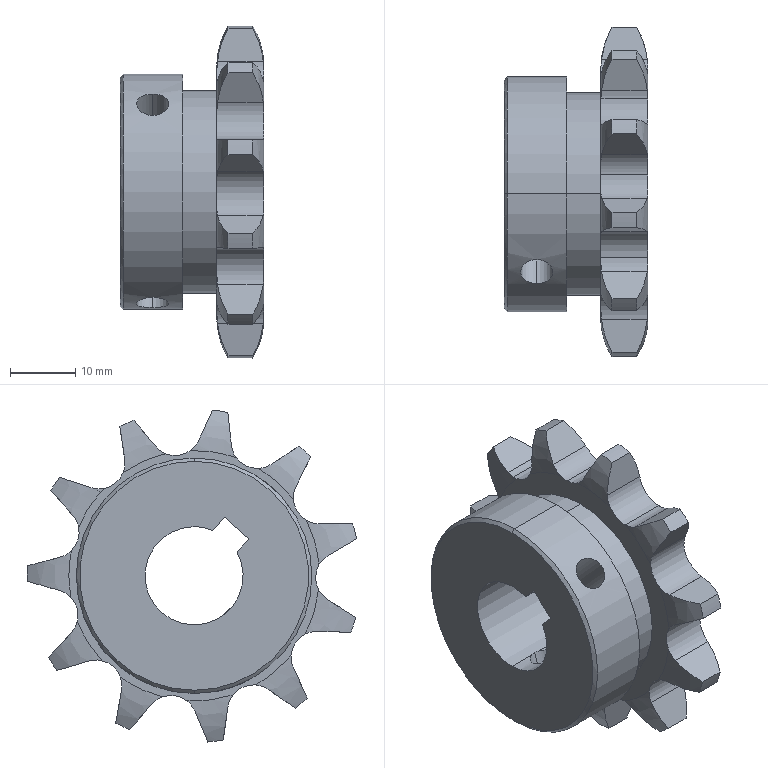Part | SolidWorks | features BaseBody 1 | 1 solid | 92 faces | box 22 x 50.358 x 50.761 mm | volume 19243 mm3 | cylinder 37 | plane 29 | spline 24 | cone 2 | commonest cylinder face diameters 7.92 x15 51 x11 4.917 x4 15 x3 31 x2 36 x2